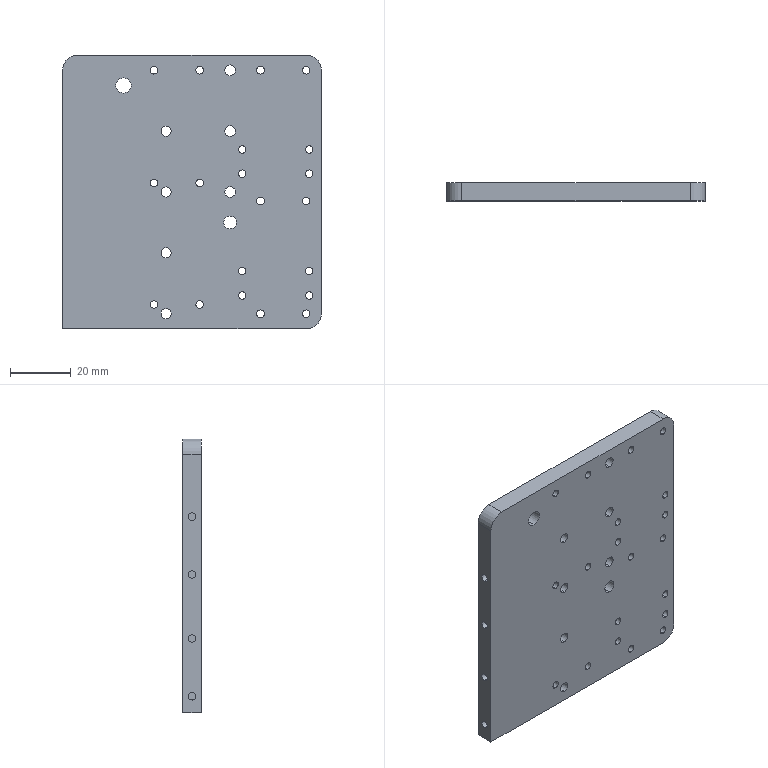Part | STEP file | 0246_202_Plate | 1 solid | 88 faces | box 85 x 6 x 90 mm | volume 44217 mm3 | cylinder 75 | plane 13 | commonest cylinder face diameters 2.5 x48 3.3 x8 3.5 x6 6.5 x6 10 x3 4.2 x2